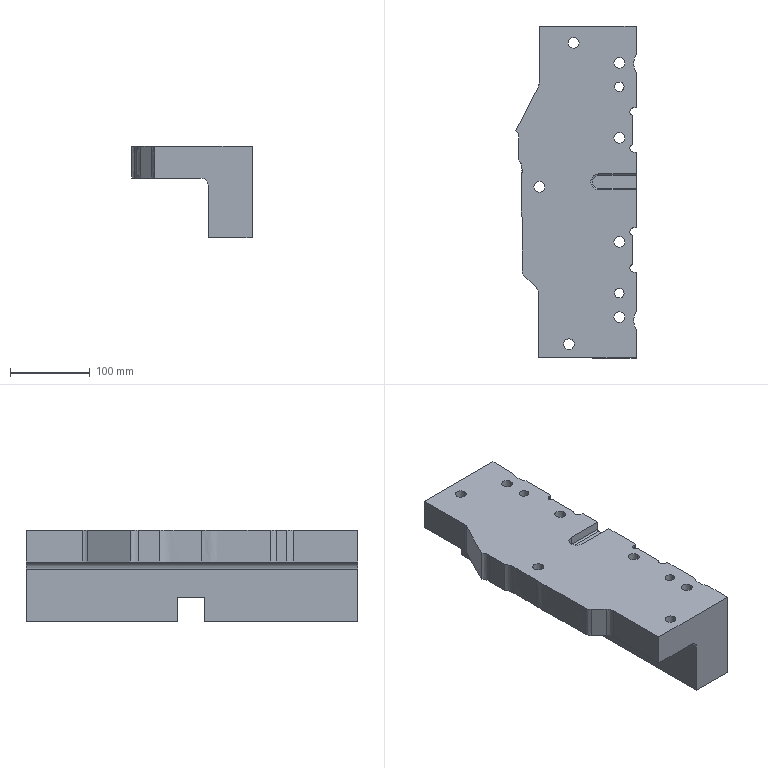Part | NX | features solid 2 | 1 solid | 112 faces | box 150.361 x 415 x 115 mm | volume 3565101 mm3 | plane 43 | cylinder 42 | cone 18 | spline 8 | torus 1 | commonest cylinder face diameters 13.507 x7 20.008 x7 10 x4 10.3 x4 16 x4 4 x2